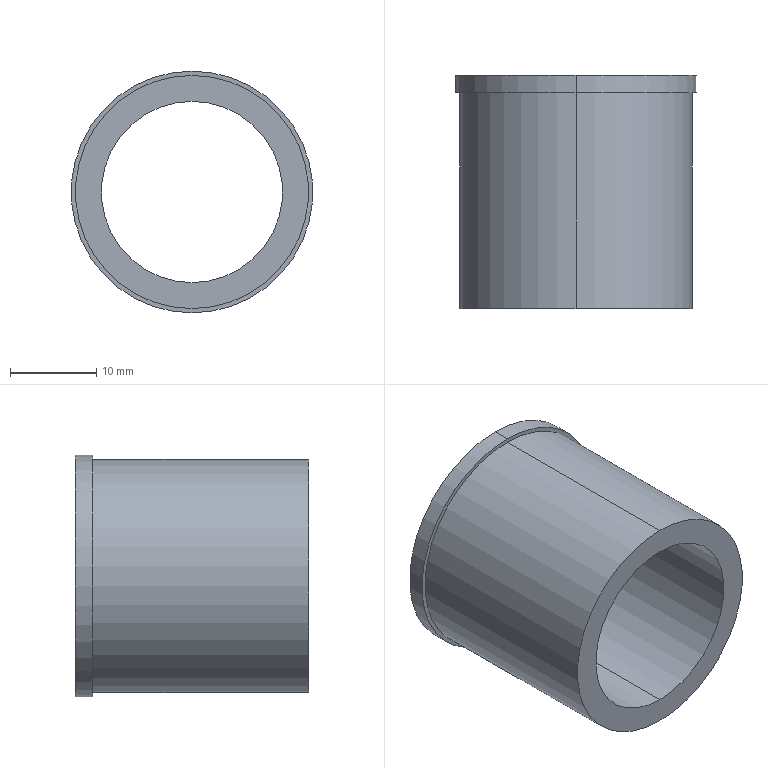Part | SolidWorks | features Revolution 1 | 1 solid | 9 faces | box 28 x 27 x 28 mm | volume 6194 mm3 | cylinder 6 | plane 3 | commonest cylinder face diameters 21 x2 27 x2 28 x2
STEP:
#1=CARTESIAN_POINT('',(0.,-2.,14.));
#2=VERTEX_POINT('',#1);
#3=CARTESIAN_POINT('',(0.,-2.,-14.));
#4=VERTEX_POINT('',#3);
#5=CARTESIAN_POINT('',(0.,-2.,0.));
#6=DIRECTION('',(0.,1.,0.));
#7=DIRECTION('',(0.,0.,1.));
#8=AXIS2_PLACEMENT_3D('',#5,#6,#7);
#9=CIRCLE('',#8,14.);
#10=EDGE_CURVE('',#2,#4,#9,.T.);
#11=ORIENTED_EDGE('',*,*,#10,.T.);
#12=CARTESIAN_POINT('',(0.,0.,-14.));
#13=VERTEX_POINT('',#12);
#14=CARTESIAN_POINT('',(0.,4.077,-14.));
#15=DIRECTION('',(0.,1.,0.));
#16=VECTOR('',#15,1000.);
#17=LINE('',#14,#16);
#18=EDGE_CURVE('',#4,#13,#17,.T.);
#19=ORIENTED_EDGE('',*,*,#18,.T.);
#20=CARTESIAN_POINT('',(0.,0.,14.));
#21=VERTEX_POINT('',#20);
#22=CARTESIAN_POINT('',(0.,0.,0.));
#23=DIRECTION('',(0.,1.,0.));
#24=DIRECTION('',(0.,0.,1.));
#25=AXIS2_PLACEMENT_3D('',#22,#23,#24);
#26=CIRCLE('',#25,14.);
#27=EDGE_CURVE('',#21,#13,#26,.T.);
#28=ORIENTED_EDGE('',*,*,#27,.F.);
#29=CARTESIAN_POINT('',(0.,4.077,14.));
#30=DIRECTION('',(0.,1.,0.));
#31=VECTOR('',#30,1000.);
#32=LINE('',#29,#31);
#33=EDGE_CURVE('',#2,#21,#32,.T.);
#34=ORIENTED_EDGE('',*,*,#33,.F.);
#35=EDGE_LOOP('',(#11,#19,#28,#34));
#36=FACE_OUTER_BOUND('',#35,.T.);
#37=CARTESIAN_POINT('',(0.,4.077,0.));
#38=DIRECTION('',(0.,1.,0.));
#39=DIRECTION('',(0.,0.,1.));
#40=AXIS2_PLACEMENT_3D('',#37,#38,#39);
#41=CYLINDRICAL_SURFACE('',#40,14.);
#42=ADVANCED_FACE('',(#36),#41,.T.);
#43=CARTESIAN_POINT('',(0.,-27.,13.5));
#44=VERTEX_POINT('',#43);
#45=CARTESIAN_POINT('',(0.,-27.,-13.5));
#46=VERTEX_POINT('',#45);
#47=CARTESIAN_POINT('',(0.,-27.,0.));
#48=DIRECTION('',(0.,1.,0.));
#49=DIRECTION('',(0.,0.,1.));
#50=AXIS2_PLACEMENT_3D('',#47,#48,#49);
#51=CIRCLE('',#50,13.5);
#52=EDGE_CURVE('',#44,#46,#51,.T.);
#53=ORIENTED_EDGE('',*,*,#52,.T.);
#54=CARTESIAN_POINT('',(0.,-2.,-13.5));
#55=VERTEX_POINT('',#54);
#56=CARTESIAN_POINT('',(0.,4.077,-13.5));
#57=DIRECTION('',(0.,1.,0.));
#58=VECTOR('',#57,1000.);
#59=LINE('',#56,#58);
#60=EDGE_CURVE('',#46,#55,#59,.T.);
#61=ORIENTED_EDGE('',*,*,#60,.T.);
#62=CARTESIAN_POINT('',(0.,-2.,13.5));
#63=VERTEX_POINT('',#62);
#64=CARTESIAN_POINT('',(0.,-2.,0.));
#65=DIRECTION('',(0.,1.,0.));
#66=DIRECTION('',(0.,0.,1.));
#67=AXIS2_PLACEMENT_3D('',#64,#65,#66);
#68=CIRCLE('',#67,13.5);
#69=EDGE_CURVE('',#63,#55,#68,.T.);
#70=ORIENTED_EDGE('',*,*,#69,.F.);
#71=CARTESIAN_POINT('',(0.,4.077,13.5));
#72=DIRECTION('',(0.,1.,0.));
#73=VECTOR('',#72,1000.);
#74=LINE('',#71,#73);
#75=EDGE_CURVE('',#44,#63,#74,.T.);
#76=ORIENTED_EDGE('',*,*,#75,.F.);
#77=EDGE_LOOP('',(#53,#61,#70,#76));
#78=FACE_OUTER_BOUND('',#77,.T.);
#79=CARTESIAN_POINT('',(0.,4.077,0.));
#80=DIRECTION('',(0.,1.,0.));
#81=DIRECTION('',(0.,0.,1.));
#82=AXIS2_PLACEMENT_3D('',#79,#80,#81);
#83=CYLINDRICAL_SURFACE('',#82,13.5);
#84=ADVANCED_FACE('',(#78),#83,.T.);
#85=CARTESIAN_POINT('',(0.,-27.,-10.5));
#86=VERTEX_POINT('',#85);
#87=CARTESIAN_POINT('',(0.,-27.,10.5));
#88=VERTEX_POINT('',#87);
#89=CARTESIAN_POINT('',(0.,-27.,0.));
#90=DIRECTION('',(0.,1.,0.));
#91=DIRECTION('',(0.,0.,1.));
#92=AXIS2_PLACEMENT_3D('',#89,#90,#91);
#93=CIRCLE('',#92,10.5);
#94=EDGE_CURVE('',#86,#88,#93,.T.);
#95=ORIENTED_EDGE('',*,*,#94,.F.);
#96=CARTESIAN_POINT('',(0.,0.,-10.5));
#97=VERTEX_POINT('',#96);
#98=CARTESIAN_POINT('',(0.,4.077,-10.5));
#99=DIRECTION('',(0.,1.,0.));
#100=VECTOR('',#99,1000.);
#101=LINE('',#98,#100);
#102=EDGE_CURVE('',#86,#97,#101,.T.);
#103=ORIENTED_EDGE('',*,*,#102,.T.);
#104=CARTESIAN_POINT('',(0.,0.,10.5));
#105=VERTEX_POINT('',#104);
#106=CARTESIAN_POINT('',(0.,0.,0.));
#107=DIRECTION('',(0.,1.,0.));
#108=DIRECTION('',(0.,0.,1.));
#109=AXIS2_PLACEMENT_3D('',#106,#107,#108);
#110=CIRCLE('',#109,10.5);
#111=EDGE_CURVE('',#97,#105,#110,.T.);
#112=ORIENTED_EDGE('',*,*,#111,.T.);
#113=CARTESIAN_POINT('',(0.,4.077,10.5));
#114=DIRECTION('',(0.,1.,0.));
#115=VECTOR('',#114,1000.);
#116=LINE('',#113,#115);
#117=EDGE_CURVE('',#88,#105,#116,.T.);
#118=ORIENTED_EDGE('',*,*,#117,.F.);
#119=EDGE_LOOP('',(#95,#103,#112,#118));
#120=FACE_OUTER_BOUND('',#119,.T.);
#121=CARTESIAN_POINT('',(0.,4.077,0.));
#122=DIRECTION('',(0.,1.,0.));
#123=DIRECTION('',(0.,0.,1.));
#124=AXIS2_PLACEMENT_3D('',#121,#122,#123);
#125=CYLINDRICAL_SURFACE('',#124,10.5);
#126=ADVANCED_FACE('',(#120),#125,.F.);
#127=ORIENTED_EDGE('',*,*,#102,.F.);
#128=CARTESIAN_POINT('',(0.,-27.,0.));
#129=DIRECTION('',(0.,1.,0.));
#130=DIRECTION('',(0.,0.,1.));
#131=AXIS2_PLACEMENT_3D('',#128,#129,#130);
#132=CIRCLE('',#131,10.5);
#133=EDGE_CURVE('',#88,#86,#132,.T.);
#134=ORIENTED_EDGE('',*,*,#133,.F.);
#135=ORIENTED_EDGE('',*,*,#117,.T.);
#136=CARTESIAN_POINT('',(0.,0.,0.));
#137=DIRECTION('',(0.,1.,0.));
#138=DIRECTION('',(0.,0.,1.));
#139=AXIS2_PLACEMENT_3D('',#136,#137,#138);
#140=CIRCLE('',#139,10.5);
#141=EDGE_CURVE('',#105,#97,#140,.T.);
#142=ORIENTED_EDGE('',*,*,#141,.T.);
#143=EDGE_LOOP('',(#127,#134,#135,#142));
#144=FACE_OUTER_BOUND('',#143,.T.);
#145=CARTESIAN_POINT('',(0.,4.077,0.));
#146=DIRECTION('',(0.,1.,0.));
#147=DIRECTION('',(0.,0.,1.));
#148=AXIS2_PLACEMENT_3D('',#145,#146,#147);
#149=CYLINDRICAL_SURFACE('',#148,10.5);
#150=ADVANCED_FACE('',(#144),#149,.F.);
#151=ORIENTED_EDGE('',*,*,#52,.F.);
#152=CARTESIAN_POINT('',(0.,-27.,0.));
#153=DIRECTION('',(0.,1.,0.));
#154=DIRECTION('',(0.,0.,1.));
#155=AXIS2_PLACEMENT_3D('',#152,#153,#154);
#156=CIRCLE('',#155,13.5);
#157=EDGE_CURVE('',#46,#44,#156,.T.);
#158=ORIENTED_EDGE('',*,*,#157,.F.);
#159=EDGE_LOOP('',(#151,#158));
#160=FACE_OUTER_BOUND('',#159,.T.);
#161=ORIENTED_EDGE('',*,*,#133,.T.);
#162=ORIENTED_EDGE('',*,*,#94,.T.);
#163=EDGE_LOOP('',(#161,#162));
#164=FACE_BOUND('',#163,.T.);
#165=CARTESIAN_POINT('',(10.5,-27.,0.));
#166=DIRECTION('',(0.,1.,0.));
#167=DIRECTION('',(0.,0.,1.));
#168=AXIS2_PLACEMENT_3D('',#165,#166,#167);
#169=PLANE('',#168);
#170=ADVANCED_FACE('',(#160,#164),#169,.F.);
#171=ORIENTED_EDGE('',*,*,#60,.F.);
#172=ORIENTED_EDGE('',*,*,#157,.T.);
#173=ORIENTED_EDGE('',*,*,#75,.T.);
#174=CARTESIAN_POINT('',(0.,-2.,0.));
#175=DIRECTION('',(0.,1.,0.));
#176=DIRECTION('',(0.,0.,1.));
#177=AXIS2_PLACEMENT_3D('',#174,#175,#176);
#178=CIRCLE('',#177,13.5);
#179=EDGE_CURVE('',#55,#63,#178,.T.);
#180=ORIENTED_EDGE('',*,*,#179,.F.);
#181=EDGE_LOOP('',(#171,#172,#173,#180));
#182=FACE_OUTER_BOUND('',#181,.T.);
#183=CARTESIAN_POINT('',(0.,4.077,0.));
#184=DIRECTION('',(0.,1.,0.));
#185=DIRECTION('',(0.,0.,1.));
#186=AXIS2_PLACEMENT_3D('',#183,#184,#185);
#187=CYLINDRICAL_SURFACE('',#186,13.5);
#188=ADVANCED_FACE('',(#182),#187,.T.);
#189=ORIENTED_EDGE('',*,*,#10,.F.);
#190=CARTESIAN_POINT('',(0.,-2.,0.));
#191=DIRECTION('',(0.,1.,0.));
#192=DIRECTION('',(0.,0.,1.));
#193=AXIS2_PLACEMENT_3D('',#190,#191,#192);
#194=CIRCLE('',#193,14.);
#195=EDGE_CURVE('',#4,#2,#194,.T.);
#196=ORIENTED_EDGE('',*,*,#195,.F.);
#197=EDGE_LOOP('',(#189,#196));
#198=FACE_OUTER_BOUND('',#197,.T.);
#199=ORIENTED_EDGE('',*,*,#69,.T.);
#200=ORIENTED_EDGE('',*,*,#179,.T.);
#201=EDGE_LOOP('',(#199,#200));
#202=FACE_BOUND('',#201,.T.);
#203=CARTESIAN_POINT('',(14.,-2.,0.));
#204=DIRECTION('',(0.,1.,0.));
#205=DIRECTION('',(0.,0.,1.));
#206=AXIS2_PLACEMENT_3D('',#203,#204,#205);
#207=PLANE('',#206);
#208=ADVANCED_FACE('',(#198,#202),#207,.F.);
#209=ORIENTED_EDGE('',*,*,#18,.F.);
#210=ORIENTED_EDGE('',*,*,#195,.T.);
#211=ORIENTED_EDGE('',*,*,#33,.T.);
#212=CARTESIAN_POINT('',(0.,0.,0.));
#213=DIRECTION('',(0.,1.,0.));
#214=DIRECTION('',(0.,0.,1.));
#215=AXIS2_PLACEMENT_3D('',#212,#213,#214);
#216=CIRCLE('',#215,14.);
#217=EDGE_CURVE('',#13,#21,#216,.T.);
#218=ORIENTED_EDGE('',*,*,#217,.F.);
#219=EDGE_LOOP('',(#209,#210,#211,#218));
#220=FACE_OUTER_BOUND('',#219,.T.);
#221=CARTESIAN_POINT('',(0.,4.077,0.));
#222=DIRECTION('',(0.,1.,0.));
#223=DIRECTION('',(0.,0.,1.));
#224=AXIS2_PLACEMENT_3D('',#221,#222,#223);
#225=CYLINDRICAL_SURFACE('',#224,14.);
#226=ADVANCED_FACE('',(#220),#225,.T.);
#227=ORIENTED_EDGE('',*,*,#141,.F.);
#228=ORIENTED_EDGE('',*,*,#111,.F.);
#229=EDGE_LOOP('',(#227,#228));
#230=FACE_BOUND('',#229,.T.);
#231=ORIENTED_EDGE('',*,*,#27,.T.);
#232=ORIENTED_EDGE('',*,*,#217,.T.);
#233=EDGE_LOOP('',(#231,#232));
#234=FACE_OUTER_BOUND('',#233,.T.);
#235=CARTESIAN_POINT('',(10.5,0.,0.));
#236=DIRECTION('',(0.,-1.,0.));
#237=DIRECTION('',(0.,0.,-1.));
#238=AXIS2_PLACEMENT_3D('',#235,#236,#237);
#239=PLANE('',#238);
#240=ADVANCED_FACE('',(#230,#234),#239,.F.);
#241=CLOSED_SHELL('',(#42,#84,#126,#150,#170,#188,#208,#226,#240));
#242=MANIFOLD_SOLID_BREP('',#241);
#243=CARTESIAN_POINT('',(0.,0.,0.));
#244=DIRECTION('',(0.,0.,1.));
#245=DIRECTION('',(1.,0.,0.));
#246=AXIS2_PLACEMENT_3D('',#243,#244,#245);
#247=(LENGTH_UNIT()NAMED_UNIT(*)SI_UNIT(.MILLI.,.METRE.));
#248=UNCERTAINTY_MEASURE_WITH_UNIT(LENGTH_MEASURE(0.00001),#247,'','');
#249=(NAMED_UNIT(*)PLANE_ANGLE_UNIT()SI_UNIT($,.RADIAN.));
#250=(NAMED_UNIT(*)SI_UNIT($,.STERADIAN.)SOLID_ANGLE_UNIT());
#251=(GEOMETRIC_REPRESENTATION_CONTEXT(3)GLOBAL_UNCERTAINTY_ASSIGNED_CONTEXT((#248))GLOBAL_UNIT_ASSIGNED_CONTEXT((#247,#249,#250))REPRESENTATION_CONTEXT('',''));
#252=ADVANCED_BREP_SHAPE_REPRESENTATION('',(#242,#246),#251);